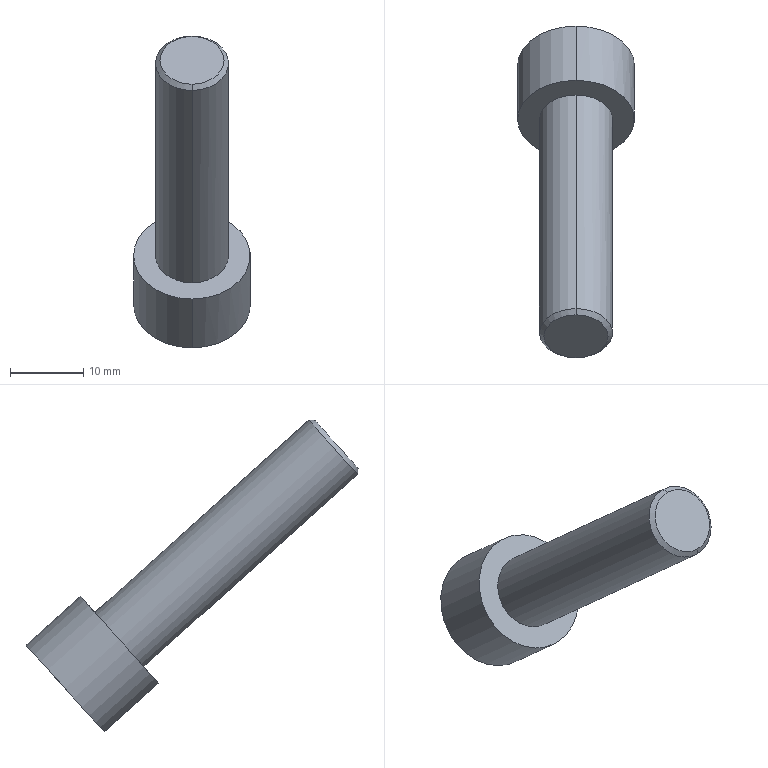Part | Creo | 1 solid | 16 faces | box 16 x 45.47 x 42.685 mm | volume 4781 mm3 | plane 10 | cylinder 4 | cone 2 | commonest cylinder face diameters 10 x2 16 x2
STEP:
#1=CARTESIAN_POINT('',(0.,0.,0.));
#2=DIRECTION('',(0.,0.,1.));
#3=DIRECTION('',(1.,0.,0.));
#4=AXIS2_PLACEMENT_3D('',#1,#2,#3);
#5=CARTESIAN_POINT('',(189.927,424.364,31.172));
#6=VERTEX_POINT('',#5);
#7=CARTESIAN_POINT('',(189.927,431.048,38.609));
#8=VERTEX_POINT('',#7);
#9=CARTESIAN_POINT('',(189.927,427.706,34.89));
#10=DIRECTION('',(0.000000011,-0.7437,0.6685));
#11=DIRECTION('',(0.,-0.6685,-0.7437));
#12=AXIS2_PLACEMENT_3D('',#9,#10,#11);
#13=CIRCLE('',#12,5.);
#14=EDGE_CURVE('',#6,#8,#13,.T.);
#15=ORIENTED_EDGE('',*,*,#14,.T.);
#16=CARTESIAN_POINT('',(189.927,460.345,12.277));
#17=VERTEX_POINT('',#16);
#18=CARTESIAN_POINT('',(189.927,460.345,12.277));
#19=DIRECTION('',(0.000000011,-0.7437,0.6685));
#20=VECTOR('',#19,39.391);
#21=LINE('',#18,#20);
#22=EDGE_CURVE('',#17,#8,#21,.T.);
#23=ORIENTED_EDGE('',*,*,#22,.F.);
#24=CARTESIAN_POINT('',(194.927,457.003,8.559));
#25=VERTEX_POINT('',#24);
#26=CARTESIAN_POINT('',(189.927,457.003,8.559));
#27=DIRECTION('',(-0.000000011,0.7437,-0.6685));
#28=DIRECTION('',(0.,0.6685,0.7437));
#29=AXIS2_PLACEMENT_3D('',#26,#27,#28);
#30=CIRCLE('',#29,5.);
#31=EDGE_CURVE('',#17,#25,#30,.T.);
#32=ORIENTED_EDGE('',*,*,#31,.T.);
#33=CARTESIAN_POINT('',(189.927,453.66,4.84));
#34=VERTEX_POINT('',#33);
#35=CARTESIAN_POINT('',(189.927,457.003,8.559));
#36=DIRECTION('',(-0.000000011,0.7437,-0.6685));
#37=DIRECTION('',(1.,0.000000015,0.));
#38=AXIS2_PLACEMENT_3D('',#35,#36,#37);
#39=CIRCLE('',#38,5.);
#40=EDGE_CURVE('',#25,#34,#39,.T.);
#41=ORIENTED_EDGE('',*,*,#40,.T.);
#42=CARTESIAN_POINT('',(189.927,453.66,4.84));
#43=DIRECTION('',(0.000000011,-0.7437,0.6685));
#44=VECTOR('',#43,39.391);
#45=LINE('',#42,#44);
#46=EDGE_CURVE('',#34,#6,#45,.T.);
#47=ORIENTED_EDGE('',*,*,#46,.T.);
#48=EDGE_LOOP('',(#15,#23,#32,#41,#47));
#49=FACE_OUTER_BOUND('',#48,.F.);
#50=CARTESIAN_POINT('',(189.927,457.003,8.559));
#51=DIRECTION('',(0.000000011,-0.7437,0.6685));
#52=DIRECTION('',(0.,-0.6685,-0.7437));
#53=AXIS2_PLACEMENT_3D('',#50,#51,#52);
#54=CYLINDRICAL_SURFACE('',#53,5.);
#55=ADVANCED_FACE('',(#49),#54,.T.);
#56=CARTESIAN_POINT('',(194.318,427.253,35.297));
#57=VERTEX_POINT('',#56);
#58=CARTESIAN_POINT('',(189.927,430.188,38.563));
#59=VERTEX_POINT('',#58);
#60=CARTESIAN_POINT('',(189.927,427.253,35.297));
#61=DIRECTION('',(0.000000011,-0.7437,0.6685));
#62=DIRECTION('',(1.,0.000000015,0.));
#63=AXIS2_PLACEMENT_3D('',#60,#61,#62);
#64=CIRCLE('',#63,4.391);
#65=EDGE_CURVE('',#57,#59,#64,.T.);
#66=ORIENTED_EDGE('',*,*,#65,.T.);
#67=CARTESIAN_POINT('',(189.927,430.188,38.563));
#68=DIRECTION('',(-0.000000008,0.9986,0.05322));
#69=VECTOR('',#68,0.8611);
#70=LINE('',#67,#69);
#71=EDGE_CURVE('',#59,#8,#70,.T.);
#72=ORIENTED_EDGE('',*,*,#71,.T.);
#73=ORIENTED_EDGE('',*,*,#14,.F.);
#74=CARTESIAN_POINT('',(189.927,424.318,32.032));
#75=VERTEX_POINT('',#74);
#76=CARTESIAN_POINT('',(189.927,424.318,32.032));
#77=DIRECTION('',(-0.000000008,0.05322,-0.9986));
#78=VECTOR('',#77,0.8611);
#79=LINE('',#76,#78);
#80=EDGE_CURVE('',#75,#6,#79,.T.);
#81=ORIENTED_EDGE('',*,*,#80,.F.);
#82=CARTESIAN_POINT('',(189.927,427.253,35.297));
#83=DIRECTION('',(0.000000011,-0.7437,0.6685));
#84=DIRECTION('',(0.,-0.6685,-0.7437));
#85=AXIS2_PLACEMENT_3D('',#82,#83,#84);
#86=CIRCLE('',#85,4.391);
#87=EDGE_CURVE('',#75,#57,#86,.T.);
#88=ORIENTED_EDGE('',*,*,#87,.T.);
#89=EDGE_LOOP('',(#66,#72,#73,#81,#88));
#90=FACE_OUTER_BOUND('',#89,.F.);
#91=CARTESIAN_POINT('',(189.927,427.48,35.094));
#92=DIRECTION('',(-0.000000011,0.7437,-0.6685));
#93=DIRECTION('',(0.,0.6685,0.7437));
#94=AXIS2_PLACEMENT_3D('',#91,#92,#93);
#95=CONICAL_SURFACE('',#94,4.696,45.);
#96=ADVANCED_FACE('',(#90),#95,.T.);
#97=CARTESIAN_POINT('',(185.536,427.253,35.297));
#98=VERTEX_POINT('',#97);
#99=CARTESIAN_POINT('',(189.927,427.253,35.297));
#100=DIRECTION('',(0.000000011,-0.7437,0.6685));
#101=DIRECTION('',(-1.,-0.000000015,0.));
#102=AXIS2_PLACEMENT_3D('',#99,#100,#101);
#103=CIRCLE('',#102,4.391);
#104=EDGE_CURVE('',#98,#75,#103,.T.);
#105=ORIENTED_EDGE('',*,*,#104,.F.);
#106=CARTESIAN_POINT('',(189.927,427.253,35.297));
#107=DIRECTION('',(0.000000011,-0.7437,0.6685));
#108=DIRECTION('',(0.,0.6685,0.7437));
#109=AXIS2_PLACEMENT_3D('',#106,#107,#108);
#110=CIRCLE('',#109,4.391);
#111=EDGE_CURVE('',#59,#98,#110,.T.);
#112=ORIENTED_EDGE('',*,*,#111,.F.);
#113=ORIENTED_EDGE('',*,*,#65,.F.);
#114=ORIENTED_EDGE('',*,*,#87,.F.);
#115=EDGE_LOOP('',(#105,#112,#113,#114));
#116=FACE_OUTER_BOUND('',#115,.F.);
#117=CARTESIAN_POINT('',(189.927,427.253,35.297));
#118=DIRECTION('',(-0.000000011,0.7437,-0.6685));
#119=DIRECTION('',(0.,0.6685,0.7437));
#120=AXIS2_PLACEMENT_3D('',#117,#118,#119);
#121=PLANE('',#120);
#122=ADVANCED_FACE('',(#116),#121,.F.);
#123=ORIENTED_EDGE('',*,*,#111,.T.);
#124=ORIENTED_EDGE('',*,*,#104,.T.);
#125=ORIENTED_EDGE('',*,*,#80,.T.);
#126=CARTESIAN_POINT('',(184.927,427.706,34.89));
#127=VERTEX_POINT('',#126);
#128=CARTESIAN_POINT('',(189.927,427.706,34.89));
#129=DIRECTION('',(0.000000011,-0.7437,0.6685));
#130=DIRECTION('',(-1.,-0.000000015,0.));
#131=AXIS2_PLACEMENT_3D('',#128,#129,#130);
#132=CIRCLE('',#131,5.);
#133=EDGE_CURVE('',#127,#6,#132,.T.);
#134=ORIENTED_EDGE('',*,*,#133,.F.);
#135=CARTESIAN_POINT('',(189.927,427.706,34.89));
#136=DIRECTION('',(0.000000011,-0.7437,0.6685));
#137=DIRECTION('',(0.,0.6685,0.7437));
#138=AXIS2_PLACEMENT_3D('',#135,#136,#137);
#139=CIRCLE('',#138,5.);
#140=EDGE_CURVE('',#8,#127,#139,.T.);
#141=ORIENTED_EDGE('',*,*,#140,.F.);
#142=ORIENTED_EDGE('',*,*,#71,.F.);
#143=EDGE_LOOP('',(#123,#124,#125,#134,#141,#142));
#144=FACE_OUTER_BOUND('',#143,.F.);
#145=CARTESIAN_POINT('',(189.927,427.48,35.094));
#146=DIRECTION('',(-0.000000011,0.7437,-0.6685));
#147=DIRECTION('',(0.,0.6685,0.7437));
#148=AXIS2_PLACEMENT_3D('',#145,#146,#147);
#149=CONICAL_SURFACE('',#148,4.696,45.);
#150=ADVANCED_FACE('',(#144),#149,.T.);
#151=ORIENTED_EDGE('',*,*,#140,.T.);
#152=ORIENTED_EDGE('',*,*,#133,.T.);
#153=ORIENTED_EDGE('',*,*,#46,.F.);
#154=CARTESIAN_POINT('',(184.927,457.003,8.559));
#155=VERTEX_POINT('',#154);
#156=CARTESIAN_POINT('',(189.927,457.003,8.559));
#157=DIRECTION('',(-0.000000011,0.7437,-0.6685));
#158=DIRECTION('',(0.,-0.6685,-0.7437));
#159=AXIS2_PLACEMENT_3D('',#156,#157,#158);
#160=CIRCLE('',#159,5.);
#161=EDGE_CURVE('',#34,#155,#160,.T.);
#162=ORIENTED_EDGE('',*,*,#161,.T.);
#163=CARTESIAN_POINT('',(189.927,457.003,8.559));
#164=DIRECTION('',(-0.000000011,0.7437,-0.6685));
#165=DIRECTION('',(-1.,-0.000000015,0.));
#166=AXIS2_PLACEMENT_3D('',#163,#164,#165);
#167=CIRCLE('',#166,5.);
#168=EDGE_CURVE('',#155,#17,#167,.T.);
#169=ORIENTED_EDGE('',*,*,#168,.T.);
#170=ORIENTED_EDGE('',*,*,#22,.T.);
#171=EDGE_LOOP('',(#151,#152,#153,#162,#169,#170));
#172=FACE_OUTER_BOUND('',#171,.F.);
#173=CARTESIAN_POINT('',(189.927,457.003,8.559));
#174=DIRECTION('',(0.000000011,-0.7437,0.6685));
#175=DIRECTION('',(0.,-0.6685,-0.7437));
#176=AXIS2_PLACEMENT_3D('',#173,#174,#175);
#177=CYLINDRICAL_SURFACE('',#176,5.);
#178=ADVANCED_FACE('',(#172),#177,.T.);
#179=CARTESIAN_POINT('',(181.927,457.003,8.559));
#180=VERTEX_POINT('',#179);
#181=CARTESIAN_POINT('',(189.927,451.655,2.609));
#182=VERTEX_POINT('',#181);
#183=CARTESIAN_POINT('',(189.927,457.003,8.559));
#184=DIRECTION('',(0.000000011,-0.7437,0.6685));
#185=DIRECTION('',(-1.,-0.000000015,0.));
#186=AXIS2_PLACEMENT_3D('',#183,#184,#185);
#187=CIRCLE('',#186,8.);
#188=EDGE_CURVE('',#180,#182,#187,.T.);
#189=ORIENTED_EDGE('',*,*,#188,.F.);
#190=CARTESIAN_POINT('',(189.927,462.35,14.509));
#191=VERTEX_POINT('',#190);
#192=CARTESIAN_POINT('',(189.927,457.003,8.559));
#193=DIRECTION('',(0.000000011,-0.7437,0.6685));
#194=DIRECTION('',(0.,0.6685,0.7437));
#195=AXIS2_PLACEMENT_3D('',#192,#193,#194);
#196=CIRCLE('',#195,8.);
#197=EDGE_CURVE('',#191,#180,#196,.T.);
#198=ORIENTED_EDGE('',*,*,#197,.F.);
#199=CARTESIAN_POINT('',(189.927,457.003,8.559));
#200=DIRECTION('',(0.000000011,-0.7437,0.6685));
#201=DIRECTION('',(0.,-0.6685,-0.7437));
#202=AXIS2_PLACEMENT_3D('',#199,#200,#201);
#203=CIRCLE('',#202,8.);
#204=EDGE_CURVE('',#182,#191,#203,.T.);
#205=ORIENTED_EDGE('',*,*,#204,.F.);
#206=EDGE_LOOP('',(#189,#198,#205));
#207=FACE_OUTER_BOUND('',#206,.F.);
#208=ORIENTED_EDGE('',*,*,#168,.F.);
#209=ORIENTED_EDGE('',*,*,#161,.F.);
#210=ORIENTED_EDGE('',*,*,#40,.F.);
#211=ORIENTED_EDGE('',*,*,#31,.F.);
#212=EDGE_LOOP('',(#208,#209,#210,#211));
#213=FACE_BOUND('',#212,.F.);
#214=CARTESIAN_POINT('',(189.927,457.003,8.559));
#215=DIRECTION('',(0.000000011,-0.7437,0.6685));
#216=DIRECTION('',(0.,-0.6685,-0.7437));
#217=AXIS2_PLACEMENT_3D('',#214,#215,#216);
#218=PLANE('',#217);
#219=ADVANCED_FACE('',(#207,#213),#218,.T.);
#220=CARTESIAN_POINT('',(189.927,459.092,-4.076));
#221=VERTEX_POINT('',#220);
#222=CARTESIAN_POINT('',(181.927,464.44,1.874));
#223=VERTEX_POINT('',#222);
#224=CARTESIAN_POINT('',(189.927,464.44,1.874));
#225=DIRECTION('',(-0.000000011,0.7437,-0.6685));
#226=DIRECTION('',(0.,-0.6685,-0.7437));
#227=AXIS2_PLACEMENT_3D('',#224,#225,#226);
#228=CIRCLE('',#227,8.);
#229=EDGE_CURVE('',#221,#223,#228,.T.);
#230=ORIENTED_EDGE('',*,*,#229,.T.);
#231=CARTESIAN_POINT('',(189.927,469.788,7.824));
#232=VERTEX_POINT('',#231);
#233=CARTESIAN_POINT('',(189.927,464.44,1.874));
#234=DIRECTION('',(-0.000000011,0.7437,-0.6685));
#235=DIRECTION('',(-1.,-0.000000015,0.));
#236=AXIS2_PLACEMENT_3D('',#233,#234,#235);
#237=CIRCLE('',#236,8.);
#238=EDGE_CURVE('',#223,#232,#237,.T.);
#239=ORIENTED_EDGE('',*,*,#238,.T.);
#240=CARTESIAN_POINT('',(189.927,462.35,14.509));
#241=DIRECTION('',(-0.000000011,0.7437,-0.6685));
#242=VECTOR('',#241,10.);
#243=LINE('',#240,#242);
#244=EDGE_CURVE('',#191,#232,#243,.T.);
#245=ORIENTED_EDGE('',*,*,#244,.F.);
#246=ORIENTED_EDGE('',*,*,#197,.T.);
#247=ORIENTED_EDGE('',*,*,#188,.T.);
#248=CARTESIAN_POINT('',(189.927,451.655,2.609));
#249=DIRECTION('',(-0.000000011,0.7437,-0.6685));
#250=VECTOR('',#249,10.);
#251=LINE('',#248,#250);
#252=EDGE_CURVE('',#182,#221,#251,.T.);
#253=ORIENTED_EDGE('',*,*,#252,.T.);
#254=EDGE_LOOP('',(#230,#239,#245,#246,#247,#253));
#255=FACE_OUTER_BOUND('',#254,.F.);
#256=CARTESIAN_POINT('',(189.927,457.003,8.559));
#257=DIRECTION('',(-0.000000011,0.7437,-0.6685));
#258=DIRECTION('',(0.,0.6685,0.7437));
#259=AXIS2_PLACEMENT_3D('',#256,#257,#258);
#260=CYLINDRICAL_SURFACE('',#259,8.);
#261=ADVANCED_FACE('',(#255),#260,.T.);
#262=ORIENTED_EDGE('',*,*,#238,.F.);
#263=ORIENTED_EDGE('',*,*,#229,.F.);
#264=CARTESIAN_POINT('',(197.927,464.44,1.874));
#265=VERTEX_POINT('',#264);
#266=CARTESIAN_POINT('',(189.927,464.44,1.874));
#267=DIRECTION('',(-0.000000011,0.7437,-0.6685));
#268=DIRECTION('',(1.,0.000000015,0.));
#269=AXIS2_PLACEMENT_3D('',#266,#267,#268);
#270=CIRCLE('',#269,8.);
#271=EDGE_CURVE('',#265,#221,#270,.T.);
#272=ORIENTED_EDGE('',*,*,#271,.F.);
#273=CARTESIAN_POINT('',(189.927,464.44,1.874));
#274=DIRECTION('',(-0.000000011,0.7437,-0.6685));
#275=DIRECTION('',(0.,0.6685,0.7437));
#276=AXIS2_PLACEMENT_3D('',#273,#274,#275);
#277=CIRCLE('',#276,8.);
#278=EDGE_CURVE('',#232,#265,#277,.T.);
#279=ORIENTED_EDGE('',*,*,#278,.F.);
#280=EDGE_LOOP('',(#262,#263,#272,#279));
#281=FACE_OUTER_BOUND('',#280,.F.);
#282=CARTESIAN_POINT('',(187.617,461.766,-1.101));
#283=VERTEX_POINT('',#282);
#284=CARTESIAN_POINT('',(192.236,461.766,-1.101));
#285=VERTEX_POINT('',#284);
#286=CARTESIAN_POINT('',(187.617,461.766,-1.101));
#287=DIRECTION('',(1.,0.000000015,0.));
#288=VECTOR('',#287,4.619);
#289=LINE('',#286,#288);
#290=EDGE_CURVE('',#283,#285,#289,.T.);
#291=ORIENTED_EDGE('',*,*,#290,.F.);
#292=CARTESIAN_POINT('',(185.308,464.44,1.874));
#293=VERTEX_POINT('',#292);
#294=CARTESIAN_POINT('',(185.308,464.44,1.874));
#295=DIRECTION('',(0.5,-0.5789,-0.6441));
#296=VECTOR('',#295,4.619);
#297=LINE('',#294,#296);
#298=EDGE_CURVE('',#293,#283,#297,.T.);
#299=ORIENTED_EDGE('',*,*,#298,.F.);
#300=CARTESIAN_POINT('',(187.617,467.114,4.849));
#301=VERTEX_POINT('',#300);
#302=CARTESIAN_POINT('',(187.617,467.114,4.849));
#303=DIRECTION('',(-0.5,-0.5789,-0.6441));
#304=VECTOR('',#303,4.619);
#305=LINE('',#302,#304);
#306=EDGE_CURVE('',#301,#293,#305,.T.);
#307=ORIENTED_EDGE('',*,*,#306,.F.);
#308=CARTESIAN_POINT('',(192.236,467.114,4.849));
#309=VERTEX_POINT('',#308);
#310=CARTESIAN_POINT('',(192.236,467.114,4.849));
#311=DIRECTION('',(-1.,-0.000000015,0.));
#312=VECTOR('',#311,4.619);
#313=LINE('',#310,#312);
#314=EDGE_CURVE('',#309,#301,#313,.T.);
#315=ORIENTED_EDGE('',*,*,#314,.F.);
#316=CARTESIAN_POINT('',(194.546,464.44,1.874));
#317=VERTEX_POINT('',#316);
#318=CARTESIAN_POINT('',(194.546,464.44,1.874));
#319=DIRECTION('',(-0.5,0.5789,0.6441));
#320=VECTOR('',#319,4.619);
#321=LINE('',#318,#320);
#322=EDGE_CURVE('',#317,#309,#321,.T.);
#323=ORIENTED_EDGE('',*,*,#322,.F.);
#324=CARTESIAN_POINT('',(192.236,461.766,-1.101));
#325=DIRECTION('',(0.5,0.5789,0.6441));
#326=VECTOR('',#325,4.619);
#327=LINE('',#324,#326);
#328=EDGE_CURVE('',#285,#317,#327,.T.);
#329=ORIENTED_EDGE('',*,*,#328,.F.);
#330=EDGE_LOOP('',(#291,#299,#307,#315,#323,#329));
#331=FACE_BOUND('',#330,.F.);
#332=CARTESIAN_POINT('',(189.927,464.44,1.874));
#333=DIRECTION('',(-0.000000011,0.7437,-0.6685));
#334=DIRECTION('',(0.,0.6685,0.7437));
#335=AXIS2_PLACEMENT_3D('',#332,#333,#334);
#336=PLANE('',#335);
#337=ADVANCED_FACE('',(#281,#331),#336,.T.);
#338=ORIENTED_EDGE('',*,*,#290,.T.);
#339=CARTESIAN_POINT('',(192.236,456.858,3.311));
#340=VERTEX_POINT('',#339);
#341=CARTESIAN_POINT('',(192.236,461.766,-1.101));
#342=DIRECTION('',(0.000000011,-0.7437,0.6685));
#343=VECTOR('',#342,6.6);
#344=LINE('',#341,#343);
#345=EDGE_CURVE('',#285,#340,#344,.T.);
#346=ORIENTED_EDGE('',*,*,#345,.T.);
#347=CARTESIAN_POINT('',(187.617,456.858,3.311));
#348=VERTEX_POINT('',#347);
#349=CARTESIAN_POINT('',(187.617,456.858,3.311));
#350=DIRECTION('',(1.,0.000000015,0.));
#351=VECTOR('',#350,4.619);
#352=LINE('',#349,#351);
#353=EDGE_CURVE('',#348,#340,#352,.T.);
#354=ORIENTED_EDGE('',*,*,#353,.F.);
#355=CARTESIAN_POINT('',(187.617,456.858,3.311));
#356=DIRECTION('',(-0.000000011,0.7437,-0.6685));
#357=VECTOR('',#356,6.6);
#358=LINE('',#355,#357);
#359=EDGE_CURVE('',#348,#283,#358,.T.);
#360=ORIENTED_EDGE('',*,*,#359,.T.);
#361=EDGE_LOOP('',(#338,#346,#354,#360));
#362=FACE_OUTER_BOUND('',#361,.F.);
#363=CARTESIAN_POINT('',(192.236,456.858,3.311));
#364=DIRECTION('',(0.00000001,-0.6685,-0.7437));
#365=DIRECTION('',(0.,0.7437,-0.6685));
#366=AXIS2_PLACEMENT_3D('',#363,#364,#365);
#367=PLANE('',#366);
#368=ADVANCED_FACE('',(#362),#367,.F.);
#369=ORIENTED_EDGE('',*,*,#328,.T.);
#370=CARTESIAN_POINT('',(194.546,459.531,6.286));
#371=VERTEX_POINT('',#370);
#372=CARTESIAN_POINT('',(194.546,464.44,1.874));
#373=DIRECTION('',(0.000000011,-0.7437,0.6685));
#374=VECTOR('',#373,6.6);
#375=LINE('',#372,#374);
#376=EDGE_CURVE('',#317,#371,#375,.T.);
#377=ORIENTED_EDGE('',*,*,#376,.T.);
#378=CARTESIAN_POINT('',(192.236,456.858,3.311));
#379=DIRECTION('',(0.5,0.5789,0.6441));
#380=VECTOR('',#379,4.619);
#381=LINE('',#378,#380);
#382=EDGE_CURVE('',#340,#371,#381,.T.);
#383=ORIENTED_EDGE('',*,*,#382,.F.);
#384=ORIENTED_EDGE('',*,*,#345,.F.);
#385=EDGE_LOOP('',(#369,#377,#383,#384));
#386=FACE_OUTER_BOUND('',#385,.F.);
#387=CARTESIAN_POINT('',(194.546,459.531,6.286));
#388=DIRECTION('',(0.866,-0.3342,-0.3719));
#389=DIRECTION('',(-0.3946,0.,-0.9189));
#390=AXIS2_PLACEMENT_3D('',#387,#388,#389);
#391=PLANE('',#390);
#392=ADVANCED_FACE('',(#386),#391,.F.);
#393=ORIENTED_EDGE('',*,*,#322,.T.);
#394=CARTESIAN_POINT('',(192.236,462.205,9.261));
#395=VERTEX_POINT('',#394);
#396=CARTESIAN_POINT('',(192.236,462.205,9.261));
#397=DIRECTION('',(-0.000000011,0.7437,-0.6685));
#398=VECTOR('',#397,6.6);
#399=LINE('',#396,#398);
#400=EDGE_CURVE('',#395,#309,#399,.T.);
#401=ORIENTED_EDGE('',*,*,#400,.F.);
#402=CARTESIAN_POINT('',(194.546,459.531,6.286));
#403=DIRECTION('',(-0.5,0.5789,0.6441));
#404=VECTOR('',#403,4.619);
#405=LINE('',#402,#404);
#406=EDGE_CURVE('',#371,#395,#405,.T.);
#407=ORIENTED_EDGE('',*,*,#406,.F.);
#408=ORIENTED_EDGE('',*,*,#376,.F.);
#409=EDGE_LOOP('',(#393,#401,#407,#408));
#410=FACE_OUTER_BOUND('',#409,.F.);
#411=CARTESIAN_POINT('',(192.236,462.205,9.261));
#412=DIRECTION('',(0.866,0.3342,0.3719));
#413=DIRECTION('',(0.3946,0.,-0.9189));
#414=AXIS2_PLACEMENT_3D('',#411,#412,#413);
#415=PLANE('',#414);
#416=ADVANCED_FACE('',(#410),#415,.F.);
#417=ORIENTED_EDGE('',*,*,#314,.T.);
#418=CARTESIAN_POINT('',(187.617,462.205,9.261));
#419=VERTEX_POINT('',#418);
#420=CARTESIAN_POINT('',(187.617,467.114,4.849));
#421=DIRECTION('',(0.000000011,-0.7437,0.6685));
#422=VECTOR('',#421,6.6);
#423=LINE('',#420,#422);
#424=EDGE_CURVE('',#301,#419,#423,.T.);
#425=ORIENTED_EDGE('',*,*,#424,.T.);
#426=CARTESIAN_POINT('',(192.236,462.205,9.261));
#427=DIRECTION('',(-1.,-0.000000015,0.));
#428=VECTOR('',#427,4.619);
#429=LINE('',#426,#428);
#430=EDGE_CURVE('',#395,#419,#429,.T.);
#431=ORIENTED_EDGE('',*,*,#430,.F.);
#432=ORIENTED_EDGE('',*,*,#400,.T.);
#433=EDGE_LOOP('',(#417,#425,#431,#432));
#434=FACE_OUTER_BOUND('',#433,.F.);
#435=CARTESIAN_POINT('',(187.617,462.205,9.261));
#436=DIRECTION('',(-0.00000001,0.6685,0.7437));
#437=DIRECTION('',(0.,-0.7437,0.6685));
#438=AXIS2_PLACEMENT_3D('',#435,#436,#437);
#439=PLANE('',#438);
#440=ADVANCED_FACE('',(#434),#439,.F.);
#441=ORIENTED_EDGE('',*,*,#306,.T.);
#442=CARTESIAN_POINT('',(185.308,459.531,6.286));
#443=VERTEX_POINT('',#442);
#444=CARTESIAN_POINT('',(185.308,464.44,1.874));
#445=DIRECTION('',(0.000000011,-0.7437,0.6685));
#446=VECTOR('',#445,6.6);
#447=LINE('',#444,#446);
#448=EDGE_CURVE('',#293,#443,#447,.T.);
#449=ORIENTED_EDGE('',*,*,#448,.T.);
#450=CARTESIAN_POINT('',(187.617,462.205,9.261));
#451=DIRECTION('',(-0.5,-0.5789,-0.6441));
#452=VECTOR('',#451,4.619);
#453=LINE('',#450,#452);
#454=EDGE_CURVE('',#419,#443,#453,.T.);
#455=ORIENTED_EDGE('',*,*,#454,.F.);
#456=ORIENTED_EDGE('',*,*,#424,.F.);
#457=EDGE_LOOP('',(#441,#449,#455,#456));
#458=FACE_OUTER_BOUND('',#457,.F.);
#459=CARTESIAN_POINT('',(185.308,459.531,6.286));
#460=DIRECTION('',(-0.866,0.3342,0.3719));
#461=DIRECTION('',(0.3946,0.,0.9189));
#462=AXIS2_PLACEMENT_3D('',#459,#460,#461);
#463=PLANE('',#462);
#464=ADVANCED_FACE('',(#458),#463,.F.);
#465=ORIENTED_EDGE('',*,*,#298,.T.);
#466=ORIENTED_EDGE('',*,*,#359,.F.);
#467=CARTESIAN_POINT('',(185.308,459.531,6.286));
#468=DIRECTION('',(0.5,-0.5789,-0.6441));
#469=VECTOR('',#468,4.619);
#470=LINE('',#467,#469);
#471=EDGE_CURVE('',#443,#348,#470,.T.);
#472=ORIENTED_EDGE('',*,*,#471,.F.);
#473=ORIENTED_EDGE('',*,*,#448,.F.);
#474=EDGE_LOOP('',(#465,#466,#472,#473));
#475=FACE_OUTER_BOUND('',#474,.F.);
#476=CARTESIAN_POINT('',(187.617,456.858,3.311));
#477=DIRECTION('',(-0.866,-0.3342,-0.3719));
#478=DIRECTION('',(-0.3946,0.,0.9189));
#479=AXIS2_PLACEMENT_3D('',#476,#477,#478);
#480=PLANE('',#479);
#481=ADVANCED_FACE('',(#475),#480,.F.);
#482=ORIENTED_EDGE('',*,*,#353,.T.);
#483=ORIENTED_EDGE('',*,*,#382,.T.);
#484=ORIENTED_EDGE('',*,*,#406,.T.);
#485=ORIENTED_EDGE('',*,*,#430,.T.);
#486=ORIENTED_EDGE('',*,*,#454,.T.);
#487=ORIENTED_EDGE('',*,*,#471,.T.);
#488=EDGE_LOOP('',(#482,#483,#484,#485,#486,#487));
#489=FACE_OUTER_BOUND('',#488,.F.);
#490=CARTESIAN_POINT('',(187.617,456.858,3.311));
#491=DIRECTION('',(-0.000000011,0.7437,-0.6685));
#492=DIRECTION('',(0.,0.6685,0.7437));
#493=AXIS2_PLACEMENT_3D('',#490,#491,#492);
#494=PLANE('',#493);
#495=ADVANCED_FACE('',(#489),#494,.T.);
#496=ORIENTED_EDGE('',*,*,#271,.T.);
#497=ORIENTED_EDGE('',*,*,#252,.F.);
#498=ORIENTED_EDGE('',*,*,#204,.T.);
#499=ORIENTED_EDGE('',*,*,#244,.T.);
#500=ORIENTED_EDGE('',*,*,#278,.T.);
#501=EDGE_LOOP('',(#496,#497,#498,#499,#500));
#502=FACE_OUTER_BOUND('',#501,.F.);
#503=CARTESIAN_POINT('',(189.927,457.003,8.559));
#504=DIRECTION('',(-0.000000011,0.7437,-0.6685));
#505=DIRECTION('',(0.,0.6685,0.7437));
#506=AXIS2_PLACEMENT_3D('',#503,#504,#505);
#507=CYLINDRICAL_SURFACE('',#506,8.);
#508=ADVANCED_FACE('',(#502),#507,.T.);
#509=CLOSED_SHELL('',(#55,#96,#122,#150,#178,#219,#261,#337,#368,#392,#416,#440,#464,#481,#495,#508));
#510=MANIFOLD_SOLID_BREP('',#509);
#511=(LENGTH_UNIT()NAMED_UNIT(*)SI_UNIT(.MILLI.,.METRE.));
#512=UNCERTAINTY_MEASURE_WITH_UNIT(LENGTH_MEASURE(0.006438),#511,'','');
#513=(NAMED_UNIT(*)PLANE_ANGLE_UNIT()SI_UNIT($,.RADIAN.));
#514=PLANE_ANGLE_MEASURE_WITH_UNIT(PLANE_ANGLE_MEASURE(0.01745),#513);
#515=(CONVERSION_BASED_UNIT('DEGREE',#514)NAMED_UNIT(*)PLANE_ANGLE_UNIT());
#516=(NAMED_UNIT(*)SI_UNIT($,.STERADIAN.)SOLID_ANGLE_UNIT());
#517=(GEOMETRIC_REPRESENTATION_CONTEXT(3)GLOBAL_UNCERTAINTY_ASSIGNED_CONTEXT((#512))GLOBAL_UNIT_ASSIGNED_CONTEXT((#511,#515,#516))REPRESENTATION_CONTEXT('',''));
#518=ADVANCED_BREP_SHAPE_REPRESENTATION('',(#4,#510),#517);